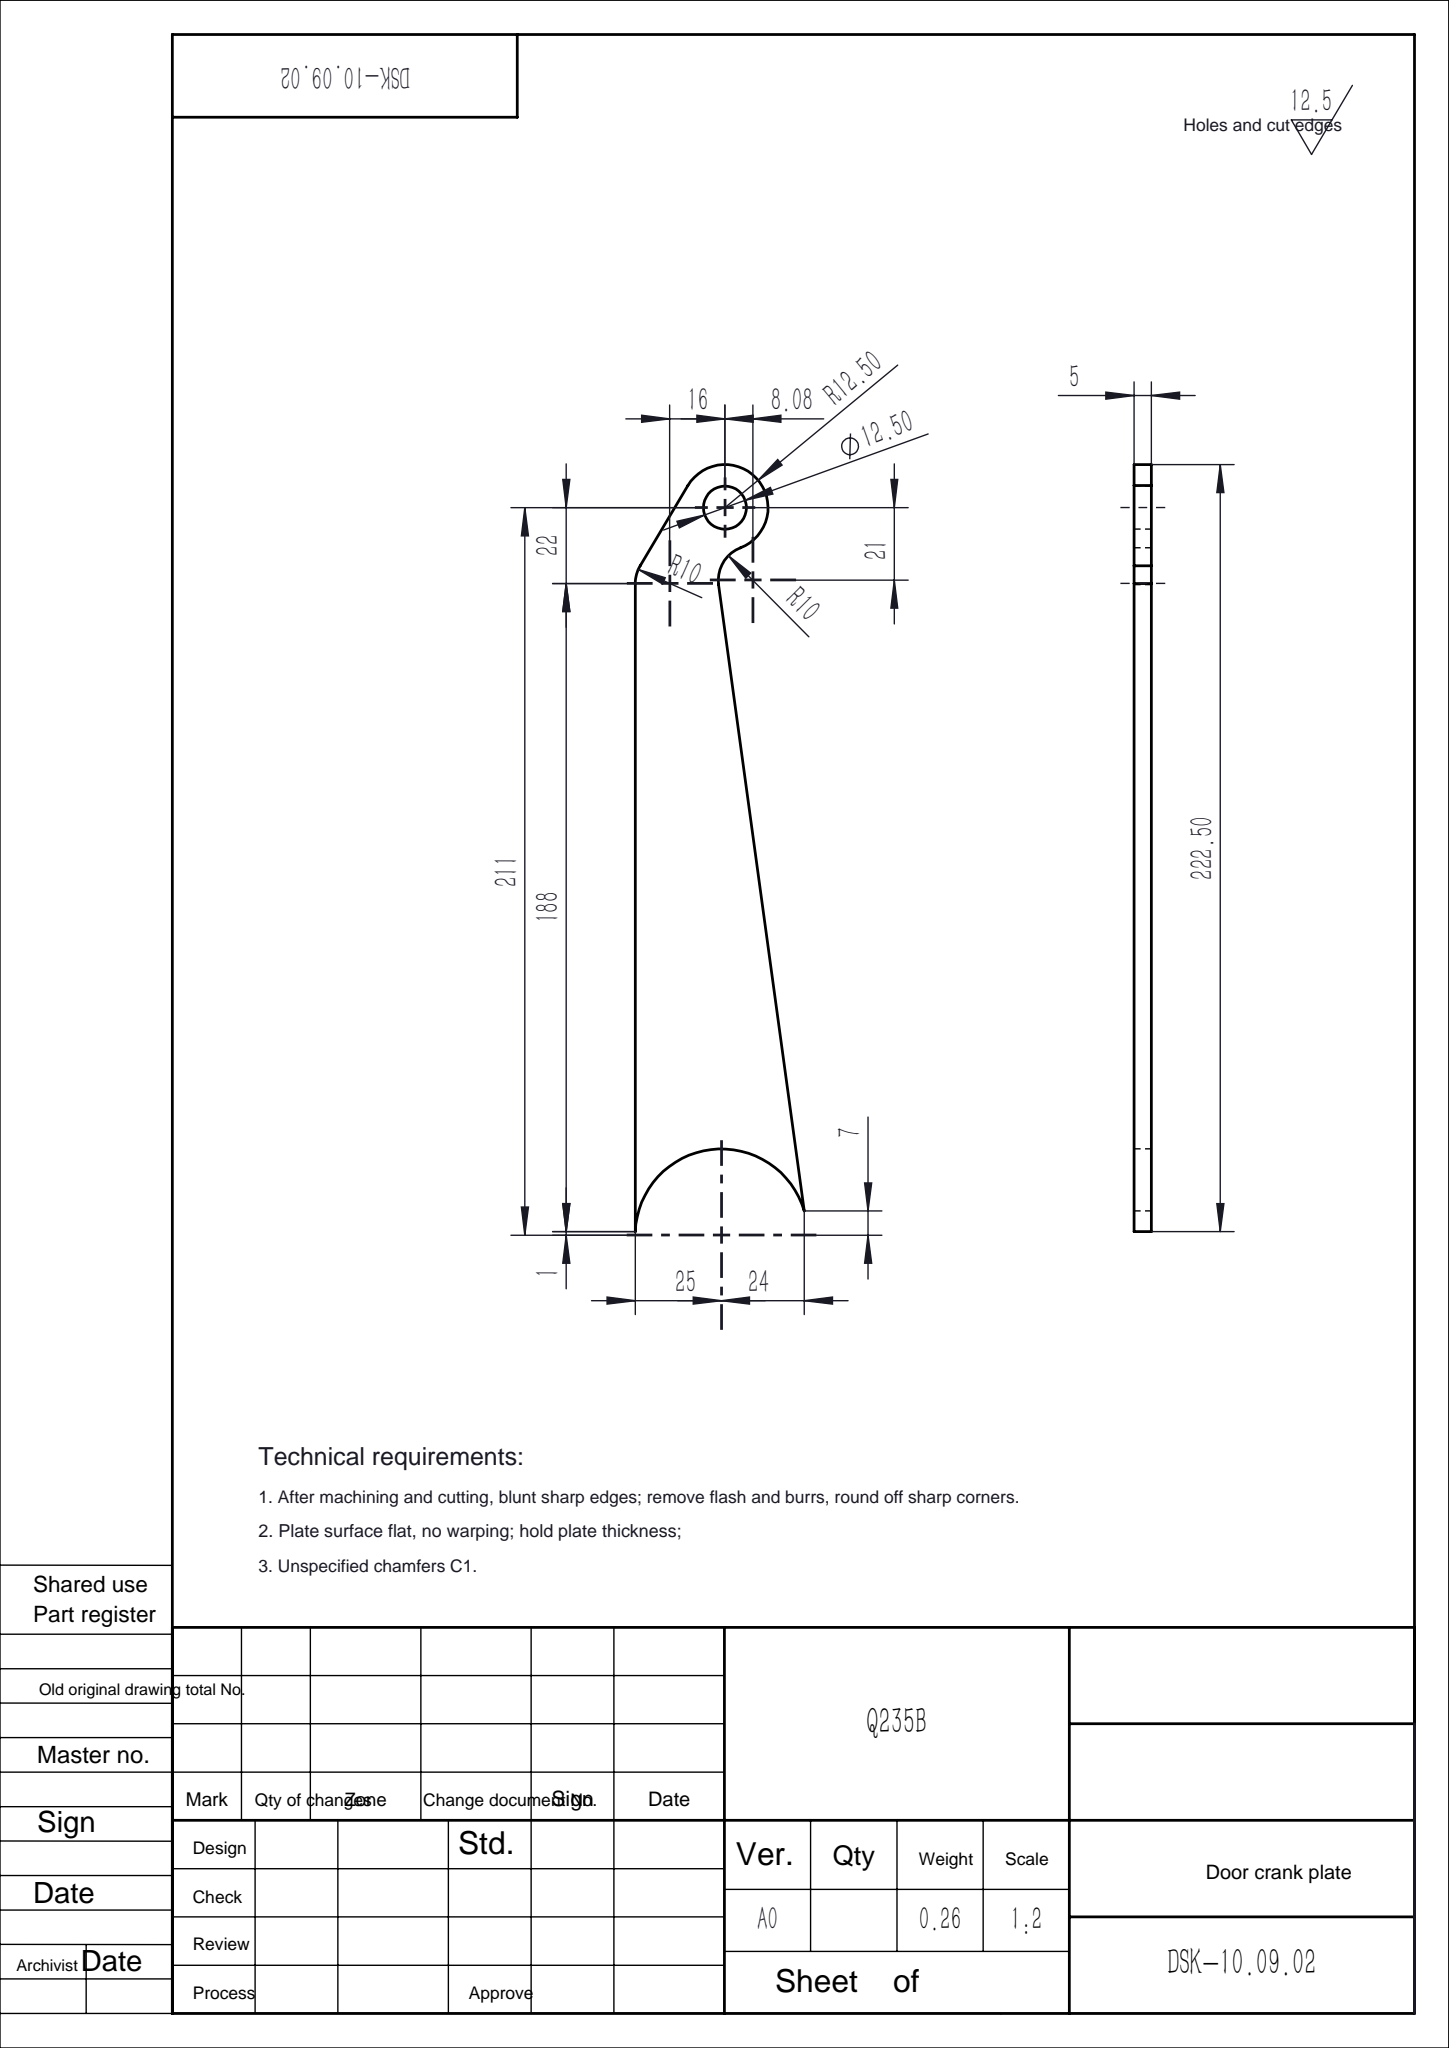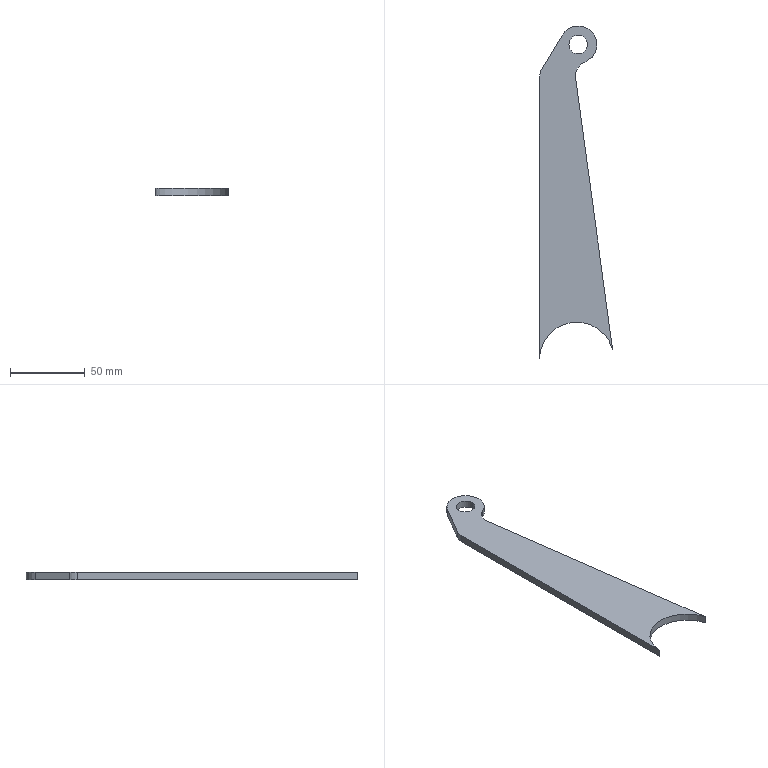Part | SolidWorks | features Extrusion 1 | 1 solid | 12 faces | box 48.98 x 222.5 x 5 mm | volume 33616 mm3 | cylinder 7 | plane 5 | commonest cylinder face diameters 20 x3 12.5 x2 25 x1 50 x1
STEP:
#1=CARTESIAN_POINT('',(-5.23,211.,5.));
#2=VERTEX_POINT('',#1);
#3=CARTESIAN_POINT('',(7.27,211.,5.));
#4=VERTEX_POINT('',#3);
#5=CARTESIAN_POINT('',(1.02,211.,5.));
#6=DIRECTION('',(0.,0.,1.));
#7=DIRECTION('',(1.,0.,0.));
#8=AXIS2_PLACEMENT_3D('',#5,#6,#7);
#9=CIRCLE('',#8,6.25);
#10=EDGE_CURVE('',#2,#4,#9,.T.);
#11=ORIENTED_EDGE('',*,*,#10,.T.);
#12=CARTESIAN_POINT('',(7.27,211.,0.));
#13=VERTEX_POINT('',#12);
#14=CARTESIAN_POINT('',(7.27,211.,5.));
#15=DIRECTION('',(0.,0.,-1.));
#16=VECTOR('',#15,1000.);
#17=LINE('',#14,#16);
#18=EDGE_CURVE('',#4,#13,#17,.T.);
#19=ORIENTED_EDGE('',*,*,#18,.T.);
#20=CARTESIAN_POINT('',(-5.23,211.,0.));
#21=VERTEX_POINT('',#20);
#22=CARTESIAN_POINT('',(1.02,211.,0.));
#23=DIRECTION('',(0.,0.,1.));
#24=DIRECTION('',(1.,0.,0.));
#25=AXIS2_PLACEMENT_3D('',#22,#23,#24);
#26=CIRCLE('',#25,6.25);
#27=EDGE_CURVE('',#21,#13,#26,.T.);
#28=ORIENTED_EDGE('',*,*,#27,.F.);
#29=CARTESIAN_POINT('',(-5.23,211.,5.));
#30=DIRECTION('',(0.,0.,-1.));
#31=VECTOR('',#30,1000.);
#32=LINE('',#29,#31);
#33=EDGE_CURVE('',#2,#21,#32,.T.);
#34=ORIENTED_EDGE('',*,*,#33,.F.);
#35=EDGE_LOOP('',(#11,#19,#28,#34));
#36=FACE_OUTER_BOUND('',#35,.T.);
#37=CARTESIAN_POINT('',(1.02,211.,5.));
#38=DIRECTION('',(0.,0.,-1.));
#39=DIRECTION('',(-1.,0.,0.));
#40=AXIS2_PLACEMENT_3D('',#37,#38,#39);
#41=CYLINDRICAL_SURFACE('',#40,6.25);
#42=ADVANCED_FACE('',(#36),#41,.F.);
#43=CARTESIAN_POINT('',(5.508,199.333,5.));
#44=VERTEX_POINT('',#43);
#45=CARTESIAN_POINT('',(-0.9022,190.,5.));
#46=VERTEX_POINT('',#45);
#47=CARTESIAN_POINT('',(9.098,190.,5.));
#48=DIRECTION('',(0.,0.,1.));
#49=DIRECTION('',(1.,0.,0.));
#50=AXIS2_PLACEMENT_3D('',#47,#48,#49);
#51=CIRCLE('',#50,10.);
#52=EDGE_CURVE('',#44,#46,#51,.T.);
#53=ORIENTED_EDGE('',*,*,#52,.T.);
#54=CARTESIAN_POINT('',(-0.9022,190.,0.));
#55=VERTEX_POINT('',#54);
#56=CARTESIAN_POINT('',(-0.9022,190.,5.));
#57=DIRECTION('',(0.,0.,-1.));
#58=VECTOR('',#57,1000.);
#59=LINE('',#56,#58);
#60=EDGE_CURVE('',#46,#55,#59,.T.);
#61=ORIENTED_EDGE('',*,*,#60,.T.);
#62=CARTESIAN_POINT('',(5.508,199.333,0.));
#63=VERTEX_POINT('',#62);
#64=CARTESIAN_POINT('',(9.098,190.,0.));
#65=DIRECTION('',(0.,0.,1.));
#66=DIRECTION('',(1.,0.,0.));
#67=AXIS2_PLACEMENT_3D('',#64,#65,#66);
#68=CIRCLE('',#67,10.);
#69=EDGE_CURVE('',#63,#55,#68,.T.);
#70=ORIENTED_EDGE('',*,*,#69,.F.);
#71=CARTESIAN_POINT('',(5.508,199.333,5.));
#72=DIRECTION('',(0.,0.,-1.));
#73=VECTOR('',#72,1000.);
#74=LINE('',#71,#73);
#75=EDGE_CURVE('',#44,#63,#74,.T.);
#76=ORIENTED_EDGE('',*,*,#75,.F.);
#77=EDGE_LOOP('',(#53,#61,#70,#76));
#78=FACE_OUTER_BOUND('',#77,.T.);
#79=CARTESIAN_POINT('',(9.098,190.,5.));
#80=DIRECTION('',(0.,0.,-1.));
#81=DIRECTION('',(-1.,0.,0.));
#82=AXIS2_PLACEMENT_3D('',#79,#80,#81);
#83=CYLINDRICAL_SURFACE('',#82,10.);
#84=ADVANCED_FACE('',(#78),#83,.F.);
#85=ORIENTED_EDGE('',*,*,#60,.F.);
#86=CARTESIAN_POINT('',(-0.8103,188.647,5.));
#87=VERTEX_POINT('',#86);
#88=CARTESIAN_POINT('',(9.098,190.,5.));
#89=DIRECTION('',(0.,0.,1.));
#90=DIRECTION('',(1.,0.,0.));
#91=AXIS2_PLACEMENT_3D('',#88,#89,#90);
#92=CIRCLE('',#91,10.);
#93=EDGE_CURVE('',#46,#87,#92,.T.);
#94=ORIENTED_EDGE('',*,*,#93,.T.);
#95=CARTESIAN_POINT('',(-0.8103,188.647,0.));
#96=VERTEX_POINT('',#95);
#97=CARTESIAN_POINT('',(-0.8103,188.647,5.));
#98=DIRECTION('',(0.,0.,-1.));
#99=VECTOR('',#98,1000.);
#100=LINE('',#97,#99);
#101=EDGE_CURVE('',#87,#96,#100,.T.);
#102=ORIENTED_EDGE('',*,*,#101,.T.);
#103=CARTESIAN_POINT('',(9.098,190.,0.));
#104=DIRECTION('',(0.,0.,1.));
#105=DIRECTION('',(1.,0.,0.));
#106=AXIS2_PLACEMENT_3D('',#103,#104,#105);
#107=CIRCLE('',#106,10.);
#108=EDGE_CURVE('',#55,#96,#107,.T.);
#109=ORIENTED_EDGE('',*,*,#108,.F.);
#110=EDGE_LOOP('',(#85,#94,#102,#109));
#111=FACE_OUTER_BOUND('',#110,.T.);
#112=CARTESIAN_POINT('',(9.098,190.,5.));
#113=DIRECTION('',(0.,0.,-1.));
#114=DIRECTION('',(-1.,0.,0.));
#115=AXIS2_PLACEMENT_3D('',#112,#113,#114);
#116=CYLINDRICAL_SURFACE('',#115,10.);
#117=ADVANCED_FACE('',(#111),#116,.F.);
#118=CARTESIAN_POINT('',(-9.722,217.392,0.));
#119=VERTEX_POINT('',#118);
#120=CARTESIAN_POINT('',(1.02,211.,0.));
#121=DIRECTION('',(0.,0.,1.));
#122=DIRECTION('',(1.,0.,0.));
#123=AXIS2_PLACEMENT_3D('',#120,#121,#122);
#124=CIRCLE('',#123,12.5);
#125=EDGE_CURVE('',#63,#119,#124,.T.);
#126=ORIENTED_EDGE('',*,*,#125,.T.);
#127=CARTESIAN_POINT('',(-9.722,217.392,5.));
#128=VERTEX_POINT('',#127);
#129=CARTESIAN_POINT('',(-9.722,217.392,5.));
#130=DIRECTION('',(0.,0.,-1.));
#131=VECTOR('',#130,1000.);
#132=LINE('',#129,#131);
#133=EDGE_CURVE('',#128,#119,#132,.T.);
#134=ORIENTED_EDGE('',*,*,#133,.F.);
#135=CARTESIAN_POINT('',(1.02,211.,5.));
#136=DIRECTION('',(0.,0.,1.));
#137=DIRECTION('',(1.,0.,0.));
#138=AXIS2_PLACEMENT_3D('',#135,#136,#137);
#139=CIRCLE('',#138,12.5);
#140=EDGE_CURVE('',#44,#128,#139,.T.);
#141=ORIENTED_EDGE('',*,*,#140,.F.);
#142=ORIENTED_EDGE('',*,*,#75,.T.);
#143=EDGE_LOOP('',(#126,#134,#141,#142));
#144=FACE_OUTER_BOUND('',#143,.T.);
#145=CARTESIAN_POINT('',(1.02,211.,5.));
#146=DIRECTION('',(0.,0.,-1.));
#147=DIRECTION('',(-1.,0.,0.));
#148=AXIS2_PLACEMENT_3D('',#145,#146,#147);
#149=CYLINDRICAL_SURFACE('',#148,12.5);
#150=ADVANCED_FACE('',(#144),#149,.T.);
#151=CARTESIAN_POINT('',(-23.574,194.114,0.));
#152=VERTEX_POINT('',#151);
#153=CARTESIAN_POINT('',(-102.712,61.118,0.));
#154=DIRECTION('',(0.5114,0.8594,0.));
#155=VECTOR('',#154,1000.);
#156=LINE('',#153,#155);
#157=EDGE_CURVE('',#152,#119,#156,.T.);
#158=ORIENTED_EDGE('',*,*,#157,.F.);
#159=CARTESIAN_POINT('',(-23.574,194.114,5.));
#160=VERTEX_POINT('',#159);
#161=CARTESIAN_POINT('',(-23.574,194.114,5.));
#162=DIRECTION('',(0.,0.,-1.));
#163=VECTOR('',#162,1000.);
#164=LINE('',#161,#163);
#165=EDGE_CURVE('',#160,#152,#164,.T.);
#166=ORIENTED_EDGE('',*,*,#165,.F.);
#167=CARTESIAN_POINT('',(-102.712,61.118,5.));
#168=DIRECTION('',(0.5114,0.8594,0.));
#169=VECTOR('',#168,1000.);
#170=LINE('',#167,#169);
#171=EDGE_CURVE('',#160,#128,#170,.T.);
#172=ORIENTED_EDGE('',*,*,#171,.T.);
#173=ORIENTED_EDGE('',*,*,#133,.T.);
#174=EDGE_LOOP('',(#158,#166,#172,#173));
#175=FACE_OUTER_BOUND('',#174,.T.);
#176=CARTESIAN_POINT('',(-102.712,61.118,5.));
#177=DIRECTION('',(-0.8594,0.5114,0.));
#178=DIRECTION('',(-0.5114,-0.8594,0.));
#179=AXIS2_PLACEMENT_3D('',#176,#177,#178);
#180=PLANE('',#179);
#181=ADVANCED_FACE('',(#175),#180,.T.);
#182=CARTESIAN_POINT('',(-24.98,189.,0.));
#183=VERTEX_POINT('',#182);
#184=CARTESIAN_POINT('',(-14.98,189.,0.));
#185=DIRECTION('',(0.,0.,1.));
#186=DIRECTION('',(1.,0.,0.));
#187=AXIS2_PLACEMENT_3D('',#184,#185,#186);
#188=CIRCLE('',#187,10.);
#189=EDGE_CURVE('',#152,#183,#188,.T.);
#190=ORIENTED_EDGE('',*,*,#189,.T.);
#191=CARTESIAN_POINT('',(-24.98,189.,5.));
#192=VERTEX_POINT('',#191);
#193=CARTESIAN_POINT('',(-24.98,189.,5.));
#194=DIRECTION('',(0.,0.,-1.));
#195=VECTOR('',#194,1000.);
#196=LINE('',#193,#195);
#197=EDGE_CURVE('',#192,#183,#196,.T.);
#198=ORIENTED_EDGE('',*,*,#197,.F.);
#199=CARTESIAN_POINT('',(-14.98,189.,5.));
#200=DIRECTION('',(0.,0.,1.));
#201=DIRECTION('',(1.,0.,0.));
#202=AXIS2_PLACEMENT_3D('',#199,#200,#201);
#203=CIRCLE('',#202,10.);
#204=EDGE_CURVE('',#160,#192,#203,.T.);
#205=ORIENTED_EDGE('',*,*,#204,.F.);
#206=ORIENTED_EDGE('',*,*,#165,.T.);
#207=EDGE_LOOP('',(#190,#198,#205,#206));
#208=FACE_OUTER_BOUND('',#207,.T.);
#209=CARTESIAN_POINT('',(-14.98,189.,5.));
#210=DIRECTION('',(0.,0.,-1.));
#211=DIRECTION('',(-1.,0.,0.));
#212=AXIS2_PLACEMENT_3D('',#209,#210,#211);
#213=CYLINDRICAL_SURFACE('',#212,10.);
#214=ADVANCED_FACE('',(#208),#213,.T.);
#215=CARTESIAN_POINT('',(-24.98,1.,0.));
#216=VERTEX_POINT('',#215);
#217=CARTESIAN_POINT('',(-24.98,0.,0.));
#218=DIRECTION('',(0.,1.,0.));
#219=VECTOR('',#218,1000.);
#220=LINE('',#217,#219);
#221=EDGE_CURVE('',#216,#183,#220,.T.);
#222=ORIENTED_EDGE('',*,*,#221,.F.);
#223=CARTESIAN_POINT('',(-24.98,1.,5.));
#224=VERTEX_POINT('',#223);
#225=CARTESIAN_POINT('',(-24.98,1.,5.));
#226=DIRECTION('',(0.,0.,-1.));
#227=VECTOR('',#226,1000.);
#228=LINE('',#225,#227);
#229=EDGE_CURVE('',#224,#216,#228,.T.);
#230=ORIENTED_EDGE('',*,*,#229,.F.);
#231=CARTESIAN_POINT('',(-24.98,0.,5.));
#232=DIRECTION('',(0.,1.,0.));
#233=VECTOR('',#232,1000.);
#234=LINE('',#231,#233);
#235=EDGE_CURVE('',#224,#192,#234,.T.);
#236=ORIENTED_EDGE('',*,*,#235,.T.);
#237=ORIENTED_EDGE('',*,*,#197,.T.);
#238=EDGE_LOOP('',(#222,#230,#236,#237));
#239=FACE_OUTER_BOUND('',#238,.T.);
#240=CARTESIAN_POINT('',(-24.98,0.,5.));
#241=DIRECTION('',(-1.,0.,0.));
#242=DIRECTION('',(0.,0.,1.));
#243=AXIS2_PLACEMENT_3D('',#240,#241,#242);
#244=PLANE('',#243);
#245=ADVANCED_FACE('',(#239),#244,.T.);
#246=CARTESIAN_POINT('',(24.,7.,0.));
#247=VERTEX_POINT('',#246);
#248=CARTESIAN_POINT('',(0.,0.,0.));
#249=DIRECTION('',(0.,0.,1.));
#250=DIRECTION('',(1.,0.,0.));
#251=AXIS2_PLACEMENT_3D('',#248,#249,#250);
#252=CIRCLE('',#251,25.);
#253=EDGE_CURVE('',#247,#216,#252,.T.);
#254=ORIENTED_EDGE('',*,*,#253,.F.);
#255=CARTESIAN_POINT('',(24.,7.,5.));
#256=VERTEX_POINT('',#255);
#257=CARTESIAN_POINT('',(24.,7.,5.));
#258=DIRECTION('',(0.,0.,-1.));
#259=VECTOR('',#258,1000.);
#260=LINE('',#257,#259);
#261=EDGE_CURVE('',#256,#247,#260,.T.);
#262=ORIENTED_EDGE('',*,*,#261,.F.);
#263=CARTESIAN_POINT('',(0.,0.,5.));
#264=DIRECTION('',(0.,0.,1.));
#265=DIRECTION('',(1.,0.,0.));
#266=AXIS2_PLACEMENT_3D('',#263,#264,#265);
#267=CIRCLE('',#266,25.);
#268=EDGE_CURVE('',#256,#224,#267,.T.);
#269=ORIENTED_EDGE('',*,*,#268,.T.);
#270=ORIENTED_EDGE('',*,*,#229,.T.);
#271=EDGE_LOOP('',(#254,#262,#269,#270));
#272=FACE_OUTER_BOUND('',#271,.T.);
#273=CARTESIAN_POINT('',(0.,0.,5.));
#274=DIRECTION('',(0.,0.,-1.));
#275=DIRECTION('',(-1.,0.,0.));
#276=AXIS2_PLACEMENT_3D('',#273,#274,#275);
#277=CYLINDRICAL_SURFACE('',#276,25.);
#278=ADVANCED_FACE('',(#272),#277,.F.);
#279=CARTESIAN_POINT('',(24.499,3.346,0.));
#280=DIRECTION('',(-0.1353,0.9908,0.));
#281=VECTOR('',#280,1000.);
#282=LINE('',#279,#281);
#283=EDGE_CURVE('',#247,#96,#282,.T.);
#284=ORIENTED_EDGE('',*,*,#283,.T.);
#285=ORIENTED_EDGE('',*,*,#101,.F.);
#286=CARTESIAN_POINT('',(24.499,3.346,5.));
#287=DIRECTION('',(-0.1353,0.9908,0.));
#288=VECTOR('',#287,1000.);
#289=LINE('',#286,#288);
#290=EDGE_CURVE('',#256,#87,#289,.T.);
#291=ORIENTED_EDGE('',*,*,#290,.F.);
#292=ORIENTED_EDGE('',*,*,#261,.T.);
#293=EDGE_LOOP('',(#284,#285,#291,#292));
#294=FACE_OUTER_BOUND('',#293,.T.);
#295=CARTESIAN_POINT('',(24.499,3.346,5.));
#296=DIRECTION('',(-0.9908,-0.1353,0.));
#297=DIRECTION('',(0.1353,-0.9908,0.));
#298=AXIS2_PLACEMENT_3D('',#295,#296,#297);
#299=PLANE('',#298);
#300=ADVANCED_FACE('',(#294),#299,.F.);
#301=ORIENTED_EDGE('',*,*,#18,.F.);
#302=CARTESIAN_POINT('',(1.02,211.,5.));
#303=DIRECTION('',(0.,0.,1.));
#304=DIRECTION('',(1.,0.,0.));
#305=AXIS2_PLACEMENT_3D('',#302,#303,#304);
#306=CIRCLE('',#305,6.25);
#307=EDGE_CURVE('',#4,#2,#306,.T.);
#308=ORIENTED_EDGE('',*,*,#307,.T.);
#309=ORIENTED_EDGE('',*,*,#33,.T.);
#310=CARTESIAN_POINT('',(1.02,211.,0.));
#311=DIRECTION('',(0.,0.,1.));
#312=DIRECTION('',(1.,0.,0.));
#313=AXIS2_PLACEMENT_3D('',#310,#311,#312);
#314=CIRCLE('',#313,6.25);
#315=EDGE_CURVE('',#13,#21,#314,.T.);
#316=ORIENTED_EDGE('',*,*,#315,.F.);
#317=EDGE_LOOP('',(#301,#308,#309,#316));
#318=FACE_OUTER_BOUND('',#317,.T.);
#319=CARTESIAN_POINT('',(1.02,211.,5.));
#320=DIRECTION('',(0.,0.,-1.));
#321=DIRECTION('',(-1.,0.,0.));
#322=AXIS2_PLACEMENT_3D('',#319,#320,#321);
#323=CYLINDRICAL_SURFACE('',#322,6.25);
#324=ADVANCED_FACE('',(#318),#323,.F.);
#325=ORIENTED_EDGE('',*,*,#52,.F.);
#326=ORIENTED_EDGE('',*,*,#140,.T.);
#327=ORIENTED_EDGE('',*,*,#171,.F.);
#328=ORIENTED_EDGE('',*,*,#204,.T.);
#329=ORIENTED_EDGE('',*,*,#235,.F.);
#330=ORIENTED_EDGE('',*,*,#268,.F.);
#331=ORIENTED_EDGE('',*,*,#290,.T.);
#332=ORIENTED_EDGE('',*,*,#93,.F.);
#333=EDGE_LOOP('',(#325,#326,#327,#328,#329,#330,#331,#332));
#334=FACE_OUTER_BOUND('',#333,.T.);
#335=ORIENTED_EDGE('',*,*,#10,.F.);
#336=ORIENTED_EDGE('',*,*,#307,.F.);
#337=EDGE_LOOP('',(#335,#336));
#338=FACE_BOUND('',#337,.T.);
#339=CARTESIAN_POINT('',(0.,0.,5.));
#340=DIRECTION('',(0.,0.,1.));
#341=DIRECTION('',(1.,0.,0.));
#342=AXIS2_PLACEMENT_3D('',#339,#340,#341);
#343=PLANE('',#342);
#344=ADVANCED_FACE('',(#334,#338),#343,.T.);
#345=ORIENTED_EDGE('',*,*,#69,.T.);
#346=ORIENTED_EDGE('',*,*,#108,.T.);
#347=ORIENTED_EDGE('',*,*,#283,.F.);
#348=ORIENTED_EDGE('',*,*,#253,.T.);
#349=ORIENTED_EDGE('',*,*,#221,.T.);
#350=ORIENTED_EDGE('',*,*,#189,.F.);
#351=ORIENTED_EDGE('',*,*,#157,.T.);
#352=ORIENTED_EDGE('',*,*,#125,.F.);
#353=EDGE_LOOP('',(#345,#346,#347,#348,#349,#350,#351,#352));
#354=FACE_OUTER_BOUND('',#353,.T.);
#355=ORIENTED_EDGE('',*,*,#27,.T.);
#356=ORIENTED_EDGE('',*,*,#315,.T.);
#357=EDGE_LOOP('',(#355,#356));
#358=FACE_BOUND('',#357,.T.);
#359=CARTESIAN_POINT('',(0.,0.,0.));
#360=DIRECTION('',(0.,0.,1.));
#361=DIRECTION('',(1.,0.,0.));
#362=AXIS2_PLACEMENT_3D('',#359,#360,#361);
#363=PLANE('',#362);
#364=ADVANCED_FACE('',(#354,#358),#363,.F.);
#365=CLOSED_SHELL('',(#42,#84,#117,#150,#181,#214,#245,#278,#300,#324,#344,#364));
#366=MANIFOLD_SOLID_BREP('',#365);
#367=CARTESIAN_POINT('',(0.,0.,0.));
#368=DIRECTION('',(0.,0.,1.));
#369=DIRECTION('',(1.,0.,0.));
#370=AXIS2_PLACEMENT_3D('',#367,#368,#369);
#371=(LENGTH_UNIT()NAMED_UNIT(*)SI_UNIT(.MILLI.,.METRE.));
#372=UNCERTAINTY_MEASURE_WITH_UNIT(LENGTH_MEASURE(0.00001),#371,'','');
#373=(NAMED_UNIT(*)PLANE_ANGLE_UNIT()SI_UNIT($,.RADIAN.));
#374=(NAMED_UNIT(*)SI_UNIT($,.STERADIAN.)SOLID_ANGLE_UNIT());
#375=(GEOMETRIC_REPRESENTATION_CONTEXT(3)GLOBAL_UNCERTAINTY_ASSIGNED_CONTEXT((#372))GLOBAL_UNIT_ASSIGNED_CONTEXT((#371,#373,#374))REPRESENTATION_CONTEXT('',''));
#376=ADVANCED_BREP_SHAPE_REPRESENTATION('',(#366,#370),#375);